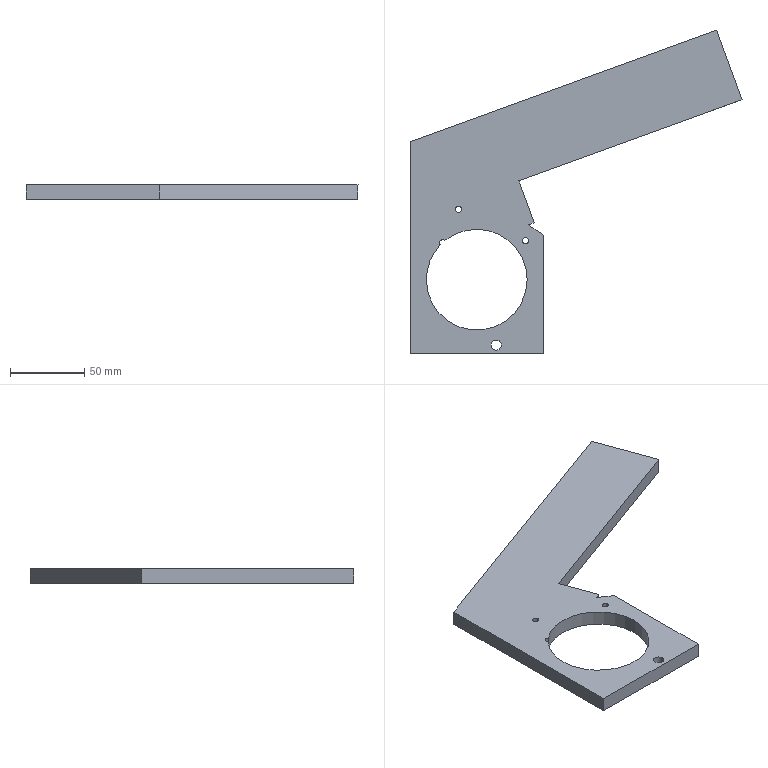Part | SolidWorks | features BaseBody 1 | 1 solid | 21 faces | box 223.833 x 218.263 x 10 mm | volume 168932 mm3 | plane 11 | cylinder 10 | commonest cylinder face diameters 4.2 x5 68 x3 6.8 x2
STEP:
#1=CARTESIAN_POINT('',(212.21,1592.079,-1033.));
#2=VERTEX_POINT('',#1);
#3=CARTESIAN_POINT('',(144.21,1592.079,-1033.));
#4=VERTEX_POINT('',#3);
#5=CARTESIAN_POINT('',(178.21,1592.079,-1033.));
#6=DIRECTION('',(0.,0.,-1.));
#7=DIRECTION('',(-1.,0.,0.));
#8=AXIS2_PLACEMENT_3D('',#5,#6,#7);
#9=CIRCLE('',#8,34.);
#10=EDGE_CURVE('',#2,#4,#9,.T.);
#11=ORIENTED_EDGE('',*,*,#10,.F.);
#12=CARTESIAN_POINT('',(212.21,1592.079,-1043.));
#13=VERTEX_POINT('',#12);
#14=CARTESIAN_POINT('',(212.21,1592.079,-936.833));
#15=DIRECTION('',(0.,0.,-1.));
#16=VECTOR('',#15,1000.);
#17=LINE('',#14,#16);
#18=EDGE_CURVE('',#2,#13,#17,.T.);
#19=ORIENTED_EDGE('',*,*,#18,.T.);
#20=CARTESIAN_POINT('',(144.21,1592.079,-1043.));
#21=VERTEX_POINT('',#20);
#22=CARTESIAN_POINT('',(178.21,1592.079,-1043.));
#23=DIRECTION('',(0.,0.,-1.));
#24=DIRECTION('',(-1.,0.,0.));
#25=AXIS2_PLACEMENT_3D('',#22,#23,#24);
#26=CIRCLE('',#25,34.);
#27=EDGE_CURVE('',#13,#21,#26,.T.);
#28=ORIENTED_EDGE('',*,*,#27,.T.);
#29=CARTESIAN_POINT('',(144.21,1592.079,-936.833));
#30=DIRECTION('',(0.,0.,-1.));
#31=VECTOR('',#30,1000.);
#32=LINE('',#29,#31);
#33=EDGE_CURVE('',#4,#21,#32,.T.);
#34=ORIENTED_EDGE('',*,*,#33,.F.);
#35=EDGE_LOOP('',(#11,#19,#28,#34));
#36=FACE_OUTER_BOUND('',#35,.T.);
#37=CARTESIAN_POINT('',(178.21,1592.079,-936.833));
#38=DIRECTION('',(0.,0.,-1.));
#39=DIRECTION('',(-1.,0.,0.));
#40=AXIS2_PLACEMENT_3D('',#37,#38,#39);
#41=CYLINDRICAL_SURFACE('',#40,34.);
#42=ADVANCED_FACE('',(#36),#41,.F.);
#43=CARTESIAN_POINT('',(153.644,1615.584,-1033.));
#44=VERTEX_POINT('',#43);
#45=CARTESIAN_POINT('',(178.21,1592.079,-1033.));
#46=DIRECTION('',(0.,0.,-1.));
#47=DIRECTION('',(-1.,0.,0.));
#48=AXIS2_PLACEMENT_3D('',#45,#46,#47);
#49=CIRCLE('',#48,34.);
#50=EDGE_CURVE('',#4,#44,#49,.T.);
#51=ORIENTED_EDGE('',*,*,#50,.F.);
#52=ORIENTED_EDGE('',*,*,#33,.T.);
#53=CARTESIAN_POINT('',(153.644,1615.584,-1043.));
#54=VERTEX_POINT('',#53);
#55=CARTESIAN_POINT('',(178.21,1592.079,-1043.));
#56=DIRECTION('',(0.,0.,-1.));
#57=DIRECTION('',(-1.,0.,0.));
#58=AXIS2_PLACEMENT_3D('',#55,#56,#57);
#59=CIRCLE('',#58,34.);
#60=EDGE_CURVE('',#21,#54,#59,.T.);
#61=ORIENTED_EDGE('',*,*,#60,.T.);
#62=CARTESIAN_POINT('',(153.644,1615.584,-1033.));
#63=DIRECTION('',(0.,0.,1.));
#64=VECTOR('',#63,1000.);
#65=LINE('',#62,#64);
#66=EDGE_CURVE('',#54,#44,#65,.T.);
#67=ORIENTED_EDGE('',*,*,#66,.T.);
#68=EDGE_LOOP('',(#51,#52,#61,#67));
#69=FACE_OUTER_BOUND('',#68,.T.);
#70=CARTESIAN_POINT('',(178.21,1592.079,-936.833));
#71=DIRECTION('',(0.,0.,-1.));
#72=DIRECTION('',(-1.,0.,0.));
#73=AXIS2_PLACEMENT_3D('',#70,#71,#72);
#74=CYLINDRICAL_SURFACE('',#73,34.);
#75=ADVANCED_FACE('',(#69),#74,.F.);
#76=CARTESIAN_POINT('',(194.715,1547.971,-1043.));
#77=VERTEX_POINT('',#76);
#78=CARTESIAN_POINT('',(187.915,1547.971,-1043.));
#79=VERTEX_POINT('',#78);
#80=CARTESIAN_POINT('',(191.315,1547.971,-1043.));
#81=DIRECTION('',(0.,0.,-1.));
#82=DIRECTION('',(1.,0.,0.));
#83=AXIS2_PLACEMENT_3D('',#80,#81,#82);
#84=CIRCLE('',#83,3.4);
#85=EDGE_CURVE('',#77,#79,#84,.T.);
#86=ORIENTED_EDGE('',*,*,#85,.T.);
#87=CARTESIAN_POINT('',(187.915,1547.971,-1033.));
#88=VERTEX_POINT('',#87);
#89=CARTESIAN_POINT('',(187.915,1547.971,-1033.));
#90=DIRECTION('',(0.,0.,1.));
#91=VECTOR('',#90,1000.);
#92=LINE('',#89,#91);
#93=EDGE_CURVE('',#79,#88,#92,.T.);
#94=ORIENTED_EDGE('',*,*,#93,.T.);
#95=CARTESIAN_POINT('',(194.715,1547.971,-1033.));
#96=VERTEX_POINT('',#95);
#97=CARTESIAN_POINT('',(191.315,1547.971,-1033.));
#98=DIRECTION('',(0.,0.,-1.));
#99=DIRECTION('',(1.,0.,0.));
#100=AXIS2_PLACEMENT_3D('',#97,#98,#99);
#101=CIRCLE('',#100,3.4);
#102=EDGE_CURVE('',#96,#88,#101,.T.);
#103=ORIENTED_EDGE('',*,*,#102,.F.);
#104=CARTESIAN_POINT('',(194.715,1547.971,-1033.));
#105=DIRECTION('',(0.,0.,1.));
#106=VECTOR('',#105,1000.);
#107=LINE('',#104,#106);
#108=EDGE_CURVE('',#77,#96,#107,.T.);
#109=ORIENTED_EDGE('',*,*,#108,.F.);
#110=EDGE_LOOP('',(#86,#94,#103,#109));
#111=FACE_OUTER_BOUND('',#110,.T.);
#112=CARTESIAN_POINT('',(191.315,1547.971,-1033.));
#113=DIRECTION('',(0.,0.,1.));
#114=DIRECTION('',(1.,0.,0.));
#115=AXIS2_PLACEMENT_3D('',#112,#113,#114);
#116=CYLINDRICAL_SURFACE('',#115,3.4);
#117=ADVANCED_FACE('',(#111),#116,.F.);
#118=CARTESIAN_POINT('',(167.934,1639.572,-1043.));
#119=VERTEX_POINT('',#118);
#120=CARTESIAN_POINT('',(163.734,1639.572,-1043.));
#121=VERTEX_POINT('',#120);
#122=CARTESIAN_POINT('',(165.834,1639.572,-1043.));
#123=DIRECTION('',(0.,0.,-1.));
#124=DIRECTION('',(1.,0.,0.));
#125=AXIS2_PLACEMENT_3D('',#122,#123,#124);
#126=CIRCLE('',#125,2.1);
#127=EDGE_CURVE('',#119,#121,#126,.T.);
#128=ORIENTED_EDGE('',*,*,#127,.T.);
#129=CARTESIAN_POINT('',(163.734,1639.572,-1033.));
#130=VERTEX_POINT('',#129);
#131=CARTESIAN_POINT('',(163.734,1639.572,-1033.));
#132=DIRECTION('',(0.,0.,1.));
#133=VECTOR('',#132,1000.);
#134=LINE('',#131,#133);
#135=EDGE_CURVE('',#121,#130,#134,.T.);
#136=ORIENTED_EDGE('',*,*,#135,.T.);
#137=CARTESIAN_POINT('',(167.934,1639.572,-1033.));
#138=VERTEX_POINT('',#137);
#139=CARTESIAN_POINT('',(165.834,1639.572,-1033.));
#140=DIRECTION('',(0.,0.,-1.));
#141=DIRECTION('',(1.,0.,0.));
#142=AXIS2_PLACEMENT_3D('',#139,#140,#141);
#143=CIRCLE('',#142,2.1);
#144=EDGE_CURVE('',#138,#130,#143,.T.);
#145=ORIENTED_EDGE('',*,*,#144,.F.);
#146=CARTESIAN_POINT('',(167.934,1639.572,-1033.));
#147=DIRECTION('',(0.,0.,1.));
#148=VECTOR('',#147,1000.);
#149=LINE('',#146,#148);
#150=EDGE_CURVE('',#119,#138,#149,.T.);
#151=ORIENTED_EDGE('',*,*,#150,.F.);
#152=EDGE_LOOP('',(#128,#136,#145,#151));
#153=FACE_OUTER_BOUND('',#152,.T.);
#154=CARTESIAN_POINT('',(165.834,1639.572,-1033.));
#155=DIRECTION('',(0.,0.,1.));
#156=DIRECTION('',(1.,0.,0.));
#157=AXIS2_PLACEMENT_3D('',#154,#155,#156);
#158=CYLINDRICAL_SURFACE('',#157,2.1);
#159=ADVANCED_FACE('',(#153),#158,.F.);
#160=CARTESIAN_POINT('',(213.25,1618.441,-1043.));
#161=VERTEX_POINT('',#160);
#162=CARTESIAN_POINT('',(209.05,1618.441,-1043.));
#163=VERTEX_POINT('',#162);
#164=CARTESIAN_POINT('',(211.15,1618.441,-1043.));
#165=DIRECTION('',(0.,0.,-1.));
#166=DIRECTION('',(1.,0.,0.));
#167=AXIS2_PLACEMENT_3D('',#164,#165,#166);
#168=CIRCLE('',#167,2.1);
#169=EDGE_CURVE('',#161,#163,#168,.T.);
#170=ORIENTED_EDGE('',*,*,#169,.T.);
#171=CARTESIAN_POINT('',(209.05,1618.441,-1033.));
#172=VERTEX_POINT('',#171);
#173=CARTESIAN_POINT('',(209.05,1618.441,-1033.));
#174=DIRECTION('',(0.,0.,1.));
#175=VECTOR('',#174,1000.);
#176=LINE('',#173,#175);
#177=EDGE_CURVE('',#163,#172,#176,.T.);
#178=ORIENTED_EDGE('',*,*,#177,.T.);
#179=CARTESIAN_POINT('',(213.25,1618.441,-1033.));
#180=VERTEX_POINT('',#179);
#181=CARTESIAN_POINT('',(211.15,1618.441,-1033.));
#182=DIRECTION('',(0.,0.,-1.));
#183=DIRECTION('',(1.,0.,0.));
#184=AXIS2_PLACEMENT_3D('',#181,#182,#183);
#185=CIRCLE('',#184,2.1);
#186=EDGE_CURVE('',#180,#172,#185,.T.);
#187=ORIENTED_EDGE('',*,*,#186,.F.);
#188=CARTESIAN_POINT('',(213.25,1618.441,-1033.));
#189=DIRECTION('',(0.,0.,1.));
#190=VECTOR('',#189,1000.);
#191=LINE('',#188,#190);
#192=EDGE_CURVE('',#161,#180,#191,.T.);
#193=ORIENTED_EDGE('',*,*,#192,.F.);
#194=EDGE_LOOP('',(#170,#178,#187,#193));
#195=FACE_OUTER_BOUND('',#194,.T.);
#196=CARTESIAN_POINT('',(211.15,1618.441,-1033.));
#197=DIRECTION('',(0.,0.,1.));
#198=DIRECTION('',(1.,0.,0.));
#199=AXIS2_PLACEMENT_3D('',#196,#197,#198);
#200=CYLINDRICAL_SURFACE('',#199,2.1);
#201=ADVANCED_FACE('',(#195),#200,.F.);
#202=CARTESIAN_POINT('',(156.724,1618.429,-1043.));
#203=VERTEX_POINT('',#202);
#204=CARTESIAN_POINT('',(178.21,1592.079,-1043.));
#205=DIRECTION('',(0.,0.,-1.));
#206=DIRECTION('',(-1.,0.,0.));
#207=AXIS2_PLACEMENT_3D('',#204,#205,#206);
#208=CIRCLE('',#207,34.);
#209=EDGE_CURVE('',#203,#13,#208,.T.);
#210=ORIENTED_EDGE('',*,*,#209,.F.);
#211=CARTESIAN_POINT('',(155.269,1616.915,-1043.));
#212=DIRECTION('',(0.,0.,-1.));
#213=DIRECTION('',(1.,0.,0.));
#214=AXIS2_PLACEMENT_3D('',#211,#212,#213);
#215=CIRCLE('',#214,2.1);
#216=EDGE_CURVE('',#54,#203,#215,.T.);
#217=ORIENTED_EDGE('',*,*,#216,.F.);
#218=ORIENTED_EDGE('',*,*,#60,.F.);
#219=ORIENTED_EDGE('',*,*,#27,.F.);
#220=EDGE_LOOP('',(#210,#217,#218,#219));
#221=FACE_BOUND('',#220,.T.);
#222=ORIENTED_EDGE('',*,*,#85,.F.);
#223=CARTESIAN_POINT('',(191.315,1547.971,-1043.));
#224=DIRECTION('',(0.,0.,-1.));
#225=DIRECTION('',(1.,0.,0.));
#226=AXIS2_PLACEMENT_3D('',#223,#224,#225);
#227=CIRCLE('',#226,3.4);
#228=EDGE_CURVE('',#79,#77,#227,.T.);
#229=ORIENTED_EDGE('',*,*,#228,.F.);
#230=EDGE_LOOP('',(#222,#229));
#231=FACE_BOUND('',#230,.T.);
#232=ORIENTED_EDGE('',*,*,#127,.F.);
#233=CARTESIAN_POINT('',(165.834,1639.572,-1043.));
#234=DIRECTION('',(0.,0.,-1.));
#235=DIRECTION('',(1.,0.,0.));
#236=AXIS2_PLACEMENT_3D('',#233,#234,#235);
#237=CIRCLE('',#236,2.1);
#238=EDGE_CURVE('',#121,#119,#237,.T.);
#239=ORIENTED_EDGE('',*,*,#238,.F.);
#240=EDGE_LOOP('',(#232,#239));
#241=FACE_BOUND('',#240,.T.);
#242=ORIENTED_EDGE('',*,*,#169,.F.);
#243=CARTESIAN_POINT('',(211.15,1618.441,-1043.));
#244=DIRECTION('',(0.,0.,-1.));
#245=DIRECTION('',(1.,0.,0.));
#246=AXIS2_PLACEMENT_3D('',#243,#244,#245);
#247=CIRCLE('',#246,2.1);
#248=EDGE_CURVE('',#163,#161,#247,.T.);
#249=ORIENTED_EDGE('',*,*,#248,.F.);
#250=EDGE_LOOP('',(#242,#249));
#251=FACE_BOUND('',#250,.T.);
#252=CARTESIAN_POINT('',(357.044,1713.357,-1043.));
#253=VERTEX_POINT('',#252);
#254=CARTESIAN_POINT('',(339.943,1760.342,-1043.));
#255=VERTEX_POINT('',#254);
#256=CARTESIAN_POINT('',(357.044,1713.357,-1043.));
#257=DIRECTION('',(-0.342,0.9397,0.));
#258=VECTOR('',#257,1000.);
#259=LINE('',#256,#258);
#260=EDGE_CURVE('',#253,#255,#259,.T.);
#261=ORIENTED_EDGE('',*,*,#260,.F.);
#262=CARTESIAN_POINT('',(206.693,1658.634,-1043.));
#263=VERTEX_POINT('',#262);
#264=CARTESIAN_POINT('',(206.693,1658.634,-1043.));
#265=DIRECTION('',(0.9397,0.342,0.));
#266=VECTOR('',#265,1000.);
#267=LINE('',#264,#266);
#268=EDGE_CURVE('',#263,#253,#267,.T.);
#269=ORIENTED_EDGE('',*,*,#268,.F.);
#270=CARTESIAN_POINT('',(216.953,1630.443,-1043.));
#271=VERTEX_POINT('',#270);
#272=CARTESIAN_POINT('',(216.953,1630.443,-1043.));
#273=DIRECTION('',(-0.342,0.9397,0.));
#274=VECTOR('',#273,1000.);
#275=LINE('',#272,#274);
#276=EDGE_CURVE('',#271,#263,#275,.T.);
#277=ORIENTED_EDGE('',*,*,#276,.F.);
#278=CARTESIAN_POINT('',(213.21,1629.081,-1043.));
#279=VERTEX_POINT('',#278);
#280=CARTESIAN_POINT('',(213.21,1629.081,-1043.));
#281=DIRECTION('',(0.9397,0.342,0.));
#282=VECTOR('',#281,1000.);
#283=LINE('',#280,#282);
#284=EDGE_CURVE('',#279,#271,#283,.T.);
#285=ORIENTED_EDGE('',*,*,#284,.F.);
#286=CARTESIAN_POINT('',(223.21,1622.079,-1043.));
#287=VERTEX_POINT('',#286);
#288=CARTESIAN_POINT('',(223.21,1622.079,-1043.));
#289=DIRECTION('',(-0.8192,0.5736,0.));
#290=VECTOR('',#289,1000.);
#291=LINE('',#288,#290);
#292=EDGE_CURVE('',#287,#279,#291,.T.);
#293=ORIENTED_EDGE('',*,*,#292,.F.);
#294=CARTESIAN_POINT('',(223.21,1542.079,-1043.));
#295=VERTEX_POINT('',#294);
#296=CARTESIAN_POINT('',(223.21,1685.097,-1043.));
#297=DIRECTION('',(0.,1.,0.));
#298=VECTOR('',#297,1000.);
#299=LINE('',#296,#298);
#300=EDGE_CURVE('',#295,#287,#299,.T.);
#301=ORIENTED_EDGE('',*,*,#300,.F.);
#302=CARTESIAN_POINT('',(133.21,1542.079,-1043.));
#303=VERTEX_POINT('',#302);
#304=CARTESIAN_POINT('',(133.21,1542.079,-1043.));
#305=DIRECTION('',(1.,0.,0.));
#306=VECTOR('',#305,1000.);
#307=LINE('',#304,#306);
#308=EDGE_CURVE('',#303,#295,#307,.T.);
#309=ORIENTED_EDGE('',*,*,#308,.F.);
#310=CARTESIAN_POINT('',(133.21,1685.097,-1043.));
#311=VERTEX_POINT('',#310);
#312=CARTESIAN_POINT('',(133.21,1685.097,-1043.));
#313=DIRECTION('',(0.,-1.,0.));
#314=VECTOR('',#313,1000.);
#315=LINE('',#312,#314);
#316=EDGE_CURVE('',#311,#303,#315,.T.);
#317=ORIENTED_EDGE('',*,*,#316,.F.);
#318=CARTESIAN_POINT('',(339.943,1760.342,-1043.));
#319=DIRECTION('',(-0.9397,-0.342,0.));
#320=VECTOR('',#319,1000.);
#321=LINE('',#318,#320);
#322=EDGE_CURVE('',#255,#311,#321,.T.);
#323=ORIENTED_EDGE('',*,*,#322,.F.);
#324=EDGE_LOOP('',(#261,#269,#277,#285,#293,#301,#309,#317,#323));
#325=FACE_OUTER_BOUND('',#324,.T.);
#326=CARTESIAN_POINT('',(133.21,1685.097,-1043.));
#327=DIRECTION('',(0.,0.,1.));
#328=DIRECTION('',(1.,0.,0.));
#329=AXIS2_PLACEMENT_3D('',#326,#327,#328);
#330=PLANE('',#329);
#331=ADVANCED_FACE('',(#221,#231,#241,#251,#325),#330,.F.);
#332=ORIENTED_EDGE('',*,*,#216,.T.);
#333=CARTESIAN_POINT('',(156.724,1618.429,-1033.));
#334=VERTEX_POINT('',#333);
#335=CARTESIAN_POINT('',(156.724,1618.429,-1033.));
#336=DIRECTION('',(0.,0.,-1.));
#337=VECTOR('',#336,1000.);
#338=LINE('',#335,#337);
#339=EDGE_CURVE('',#334,#203,#338,.T.);
#340=ORIENTED_EDGE('',*,*,#339,.F.);
#341=CARTESIAN_POINT('',(155.269,1616.915,-1033.));
#342=DIRECTION('',(0.,0.,-1.));
#343=DIRECTION('',(1.,0.,0.));
#344=AXIS2_PLACEMENT_3D('',#341,#342,#343);
#345=CIRCLE('',#344,2.1);
#346=EDGE_CURVE('',#44,#334,#345,.T.);
#347=ORIENTED_EDGE('',*,*,#346,.F.);
#348=ORIENTED_EDGE('',*,*,#66,.F.);
#349=EDGE_LOOP('',(#332,#340,#347,#348));
#350=FACE_OUTER_BOUND('',#349,.T.);
#351=CARTESIAN_POINT('',(155.269,1616.915,-1033.));
#352=DIRECTION('',(0.,0.,1.));
#353=DIRECTION('',(1.,0.,0.));
#354=AXIS2_PLACEMENT_3D('',#351,#352,#353);
#355=CYLINDRICAL_SURFACE('',#354,2.1);
#356=ADVANCED_FACE('',(#350),#355,.F.);
#357=ORIENTED_EDGE('',*,*,#18,.F.);
#358=CARTESIAN_POINT('',(178.21,1592.079,-1033.));
#359=DIRECTION('',(0.,0.,-1.));
#360=DIRECTION('',(-1.,0.,0.));
#361=AXIS2_PLACEMENT_3D('',#358,#359,#360);
#362=CIRCLE('',#361,34.);
#363=EDGE_CURVE('',#334,#2,#362,.T.);
#364=ORIENTED_EDGE('',*,*,#363,.F.);
#365=ORIENTED_EDGE('',*,*,#339,.T.);
#366=ORIENTED_EDGE('',*,*,#209,.T.);
#367=EDGE_LOOP('',(#357,#364,#365,#366));
#368=FACE_OUTER_BOUND('',#367,.T.);
#369=CARTESIAN_POINT('',(178.21,1592.079,-936.833));
#370=DIRECTION('',(0.,0.,-1.));
#371=DIRECTION('',(-1.,0.,0.));
#372=AXIS2_PLACEMENT_3D('',#369,#370,#371);
#373=CYLINDRICAL_SURFACE('',#372,34.);
#374=ADVANCED_FACE('',(#368),#373,.F.);
#375=ORIENTED_EDGE('',*,*,#93,.F.);
#376=ORIENTED_EDGE('',*,*,#228,.T.);
#377=ORIENTED_EDGE('',*,*,#108,.T.);
#378=CARTESIAN_POINT('',(191.315,1547.971,-1033.));
#379=DIRECTION('',(0.,0.,-1.));
#380=DIRECTION('',(1.,0.,0.));
#381=AXIS2_PLACEMENT_3D('',#378,#379,#380);
#382=CIRCLE('',#381,3.4);
#383=EDGE_CURVE('',#88,#96,#382,.T.);
#384=ORIENTED_EDGE('',*,*,#383,.F.);
#385=EDGE_LOOP('',(#375,#376,#377,#384));
#386=FACE_OUTER_BOUND('',#385,.T.);
#387=CARTESIAN_POINT('',(191.315,1547.971,-1033.));
#388=DIRECTION('',(0.,0.,1.));
#389=DIRECTION('',(1.,0.,0.));
#390=AXIS2_PLACEMENT_3D('',#387,#388,#389);
#391=CYLINDRICAL_SURFACE('',#390,3.4);
#392=ADVANCED_FACE('',(#386),#391,.F.);
#393=ORIENTED_EDGE('',*,*,#135,.F.);
#394=ORIENTED_EDGE('',*,*,#238,.T.);
#395=ORIENTED_EDGE('',*,*,#150,.T.);
#396=CARTESIAN_POINT('',(165.834,1639.572,-1033.));
#397=DIRECTION('',(0.,0.,-1.));
#398=DIRECTION('',(1.,0.,0.));
#399=AXIS2_PLACEMENT_3D('',#396,#397,#398);
#400=CIRCLE('',#399,2.1);
#401=EDGE_CURVE('',#130,#138,#400,.T.);
#402=ORIENTED_EDGE('',*,*,#401,.F.);
#403=EDGE_LOOP('',(#393,#394,#395,#402));
#404=FACE_OUTER_BOUND('',#403,.T.);
#405=CARTESIAN_POINT('',(165.834,1639.572,-1033.));
#406=DIRECTION('',(0.,0.,1.));
#407=DIRECTION('',(1.,0.,0.));
#408=AXIS2_PLACEMENT_3D('',#405,#406,#407);
#409=CYLINDRICAL_SURFACE('',#408,2.1);
#410=ADVANCED_FACE('',(#404),#409,.F.);
#411=ORIENTED_EDGE('',*,*,#177,.F.);
#412=ORIENTED_EDGE('',*,*,#248,.T.);
#413=ORIENTED_EDGE('',*,*,#192,.T.);
#414=CARTESIAN_POINT('',(211.15,1618.441,-1033.));
#415=DIRECTION('',(0.,0.,-1.));
#416=DIRECTION('',(1.,0.,0.));
#417=AXIS2_PLACEMENT_3D('',#414,#415,#416);
#418=CIRCLE('',#417,2.1);
#419=EDGE_CURVE('',#172,#180,#418,.T.);
#420=ORIENTED_EDGE('',*,*,#419,.F.);
#421=EDGE_LOOP('',(#411,#412,#413,#420));
#422=FACE_OUTER_BOUND('',#421,.T.);
#423=CARTESIAN_POINT('',(211.15,1618.441,-1033.));
#424=DIRECTION('',(0.,0.,1.));
#425=DIRECTION('',(1.,0.,0.));
#426=AXIS2_PLACEMENT_3D('',#423,#424,#425);
#427=CYLINDRICAL_SURFACE('',#426,2.1);
#428=ADVANCED_FACE('',(#422),#427,.F.);
#429=ORIENTED_EDGE('',*,*,#322,.T.);
#430=CARTESIAN_POINT('',(133.21,1685.097,-1033.));
#431=VERTEX_POINT('',#430);
#432=CARTESIAN_POINT('',(133.21,1685.097,-933.));
#433=DIRECTION('',(0.,0.,1.));
#434=VECTOR('',#433,1000.);
#435=LINE('',#432,#434);
#436=EDGE_CURVE('',#311,#431,#435,.T.);
#437=ORIENTED_EDGE('',*,*,#436,.T.);
#438=CARTESIAN_POINT('',(339.943,1760.342,-1033.));
#439=VERTEX_POINT('',#438);
#440=CARTESIAN_POINT('',(133.21,1685.097,-1033.));
#441=DIRECTION('',(0.9397,0.342,0.));
#442=VECTOR('',#441,1000.);
#443=LINE('',#440,#442);
#444=EDGE_CURVE('',#431,#439,#443,.T.);
#445=ORIENTED_EDGE('',*,*,#444,.T.);
#446=CARTESIAN_POINT('',(339.943,1760.342,-933.));
#447=DIRECTION('',(0.,0.,-1.));
#448=VECTOR('',#447,1000.);
#449=LINE('',#446,#448);
#450=EDGE_CURVE('',#439,#255,#449,.T.);
#451=ORIENTED_EDGE('',*,*,#450,.T.);
#452=EDGE_LOOP('',(#429,#437,#445,#451));
#453=FACE_OUTER_BOUND('',#452,.T.);
#454=CARTESIAN_POINT('',(133.21,1685.097,-933.));
#455=DIRECTION('',(-0.342,0.9397,0.));
#456=DIRECTION('',(-0.9397,-0.342,0.));
#457=AXIS2_PLACEMENT_3D('',#454,#455,#456);
#458=PLANE('',#457);
#459=ADVANCED_FACE('',(#453),#458,.T.);
#460=ORIENTED_EDGE('',*,*,#260,.T.);
#461=ORIENTED_EDGE('',*,*,#450,.F.);
#462=CARTESIAN_POINT('',(357.044,1713.357,-1033.));
#463=VERTEX_POINT('',#462);
#464=CARTESIAN_POINT('',(339.943,1760.342,-1033.));
#465=DIRECTION('',(0.342,-0.9397,0.));
#466=VECTOR('',#465,1000.);
#467=LINE('',#464,#466);
#468=EDGE_CURVE('',#439,#463,#467,.T.);
#469=ORIENTED_EDGE('',*,*,#468,.T.);
#470=CARTESIAN_POINT('',(357.044,1713.357,-865.369));
#471=DIRECTION('',(0.,0.,-1.));
#472=VECTOR('',#471,1000.);
#473=LINE('',#470,#472);
#474=EDGE_CURVE('',#463,#253,#473,.T.);
#475=ORIENTED_EDGE('',*,*,#474,.T.);
#476=EDGE_LOOP('',(#460,#461,#469,#475));
#477=FACE_OUTER_BOUND('',#476,.T.);
#478=CARTESIAN_POINT('',(339.943,1760.342,-865.369));
#479=DIRECTION('',(0.9397,0.342,0.));
#480=DIRECTION('',(-0.342,0.9397,0.));
#481=AXIS2_PLACEMENT_3D('',#478,#479,#480);
#482=PLANE('',#481);
#483=ADVANCED_FACE('',(#477),#482,.T.);
#484=ORIENTED_EDGE('',*,*,#268,.T.);
#485=ORIENTED_EDGE('',*,*,#474,.F.);
#486=CARTESIAN_POINT('',(206.693,1658.634,-1033.));
#487=VERTEX_POINT('',#486);
#488=CARTESIAN_POINT('',(206.693,1658.634,-1033.));
#489=DIRECTION('',(-0.9397,-0.342,0.));
#490=VECTOR('',#489,1000.);
#491=LINE('',#488,#490);
#492=EDGE_CURVE('',#463,#487,#491,.T.);
#493=ORIENTED_EDGE('',*,*,#492,.T.);
#494=CARTESIAN_POINT('',(206.693,1658.634,-865.369));
#495=DIRECTION('',(0.,0.,-1.));
#496=VECTOR('',#495,1000.);
#497=LINE('',#494,#496);
#498=EDGE_CURVE('',#487,#263,#497,.T.);
#499=ORIENTED_EDGE('',*,*,#498,.T.);
#500=EDGE_LOOP('',(#484,#485,#493,#499));
#501=FACE_OUTER_BOUND('',#500,.T.);
#502=CARTESIAN_POINT('',(206.693,1658.634,-865.369));
#503=DIRECTION('',(0.342,-0.9397,0.));
#504=DIRECTION('',(0.9397,0.342,0.));
#505=AXIS2_PLACEMENT_3D('',#502,#503,#504);
#506=PLANE('',#505);
#507=ADVANCED_FACE('',(#501),#506,.T.);
#508=ORIENTED_EDGE('',*,*,#276,.T.);
#509=ORIENTED_EDGE('',*,*,#498,.F.);
#510=CARTESIAN_POINT('',(216.953,1630.443,-1033.));
#511=VERTEX_POINT('',#510);
#512=CARTESIAN_POINT('',(216.953,1630.443,-1033.));
#513=DIRECTION('',(0.342,-0.9397,0.));
#514=VECTOR('',#513,1000.);
#515=LINE('',#512,#514);
#516=EDGE_CURVE('',#487,#511,#515,.T.);
#517=ORIENTED_EDGE('',*,*,#516,.T.);
#518=CARTESIAN_POINT('',(216.953,1630.443,-933.));
#519=DIRECTION('',(0.,0.,-1.));
#520=VECTOR('',#519,1000.);
#521=LINE('',#518,#520);
#522=EDGE_CURVE('',#511,#271,#521,.T.);
#523=ORIENTED_EDGE('',*,*,#522,.T.);
#524=EDGE_LOOP('',(#508,#509,#517,#523));
#525=FACE_OUTER_BOUND('',#524,.T.);
#526=CARTESIAN_POINT('',(216.953,1630.443,-933.));
#527=DIRECTION('',(0.9397,0.342,0.));
#528=DIRECTION('',(-0.342,0.9397,0.));
#529=AXIS2_PLACEMENT_3D('',#526,#527,#528);
#530=PLANE('',#529);
#531=ADVANCED_FACE('',(#525),#530,.T.);
#532=CARTESIAN_POINT('',(213.21,1629.081,-1033.));
#533=VERTEX_POINT('',#532);
#534=CARTESIAN_POINT('',(194.267,1622.186,-1033.));
#535=DIRECTION('',(-0.9397,-0.342,0.));
#536=VECTOR('',#535,1000.);
#537=LINE('',#534,#536);
#538=EDGE_CURVE('',#511,#533,#537,.T.);
#539=ORIENTED_EDGE('',*,*,#538,.T.);
#540=CARTESIAN_POINT('',(213.21,1629.081,-933.));
#541=DIRECTION('',(0.,0.,-1.));
#542=VECTOR('',#541,1000.);
#543=LINE('',#540,#542);
#544=EDGE_CURVE('',#533,#279,#543,.T.);
#545=ORIENTED_EDGE('',*,*,#544,.T.);
#546=ORIENTED_EDGE('',*,*,#284,.T.);
#547=ORIENTED_EDGE('',*,*,#522,.F.);
#548=EDGE_LOOP('',(#539,#545,#546,#547));
#549=FACE_OUTER_BOUND('',#548,.T.);
#550=CARTESIAN_POINT('',(194.267,1622.186,-933.));
#551=DIRECTION('',(0.342,-0.9397,0.));
#552=DIRECTION('',(0.9397,0.342,0.));
#553=AXIS2_PLACEMENT_3D('',#550,#551,#552);
#554=PLANE('',#553);
#555=ADVANCED_FACE('',(#549),#554,.T.);
#556=CARTESIAN_POINT('',(223.21,1622.079,-1033.));
#557=VERTEX_POINT('',#556);
#558=CARTESIAN_POINT('',(223.21,1622.079,-1033.));
#559=DIRECTION('',(-0.8192,0.5736,0.));
#560=VECTOR('',#559,1000.);
#561=LINE('',#558,#560);
#562=EDGE_CURVE('',#557,#533,#561,.T.);
#563=ORIENTED_EDGE('',*,*,#562,.F.);
#564=CARTESIAN_POINT('',(223.21,1622.079,-1043.));
#565=DIRECTION('',(0.,0.,1.));
#566=VECTOR('',#565,1000.);
#567=LINE('',#564,#566);
#568=EDGE_CURVE('',#287,#557,#567,.T.);
#569=ORIENTED_EDGE('',*,*,#568,.F.);
#570=ORIENTED_EDGE('',*,*,#292,.T.);
#571=ORIENTED_EDGE('',*,*,#544,.F.);
#572=EDGE_LOOP('',(#563,#569,#570,#571));
#573=FACE_OUTER_BOUND('',#572,.T.);
#574=CARTESIAN_POINT('',(223.21,1622.079,-1043.));
#575=DIRECTION('',(-0.5736,-0.8192,0.));
#576=DIRECTION('',(0.8192,-0.5736,0.));
#577=AXIS2_PLACEMENT_3D('',#574,#575,#576);
#578=PLANE('',#577);
#579=ADVANCED_FACE('',(#573),#578,.F.);
#580=ORIENTED_EDGE('',*,*,#300,.T.);
#581=ORIENTED_EDGE('',*,*,#568,.T.);
#582=CARTESIAN_POINT('',(223.21,1542.079,-1033.));
#583=VERTEX_POINT('',#582);
#584=CARTESIAN_POINT('',(223.21,1622.079,-1033.));
#585=DIRECTION('',(0.,1.,0.));
#586=VECTOR('',#585,1000.);
#587=LINE('',#584,#586);
#588=EDGE_CURVE('',#583,#557,#587,.T.);
#589=ORIENTED_EDGE('',*,*,#588,.F.);
#590=CARTESIAN_POINT('',(223.21,1542.079,-1043.));
#591=DIRECTION('',(0.,0.,1.));
#592=VECTOR('',#591,1000.);
#593=LINE('',#590,#592);
#594=EDGE_CURVE('',#295,#583,#593,.T.);
#595=ORIENTED_EDGE('',*,*,#594,.F.);
#596=EDGE_LOOP('',(#580,#581,#589,#595));
#597=FACE_OUTER_BOUND('',#596,.T.);
#598=CARTESIAN_POINT('',(223.21,1622.079,-1043.));
#599=DIRECTION('',(-1.,0.,0.));
#600=DIRECTION('',(0.,0.,1.));
#601=AXIS2_PLACEMENT_3D('',#598,#599,#600);
#602=PLANE('',#601);
#603=ADVANCED_FACE('',(#597),#602,.F.);
#604=ORIENTED_EDGE('',*,*,#308,.T.);
#605=ORIENTED_EDGE('',*,*,#594,.T.);
#606=CARTESIAN_POINT('',(133.21,1542.079,-1033.));
#607=VERTEX_POINT('',#606);
#608=CARTESIAN_POINT('',(223.21,1542.079,-1033.));
#609=DIRECTION('',(1.,0.,0.));
#610=VECTOR('',#609,1000.);
#611=LINE('',#608,#610);
#612=EDGE_CURVE('',#607,#583,#611,.T.);
#613=ORIENTED_EDGE('',*,*,#612,.F.);
#614=CARTESIAN_POINT('',(133.21,1542.079,-1043.));
#615=DIRECTION('',(0.,0.,1.));
#616=VECTOR('',#615,1000.);
#617=LINE('',#614,#616);
#618=EDGE_CURVE('',#303,#607,#617,.T.);
#619=ORIENTED_EDGE('',*,*,#618,.F.);
#620=EDGE_LOOP('',(#604,#605,#613,#619));
#621=FACE_OUTER_BOUND('',#620,.T.);
#622=CARTESIAN_POINT('',(223.21,1542.079,-1043.));
#623=DIRECTION('',(0.,1.,0.));
#624=DIRECTION('',(0.,0.,1.));
#625=AXIS2_PLACEMENT_3D('',#622,#623,#624);
#626=PLANE('',#625);
#627=ADVANCED_FACE('',(#621),#626,.F.);
#628=ORIENTED_EDGE('',*,*,#316,.T.);
#629=ORIENTED_EDGE('',*,*,#618,.T.);
#630=CARTESIAN_POINT('',(133.21,1685.097,-1033.));
#631=DIRECTION('',(0.,-1.,0.));
#632=VECTOR('',#631,1000.);
#633=LINE('',#630,#632);
#634=EDGE_CURVE('',#431,#607,#633,.T.);
#635=ORIENTED_EDGE('',*,*,#634,.F.);
#636=ORIENTED_EDGE('',*,*,#436,.F.);
#637=EDGE_LOOP('',(#628,#629,#635,#636));
#638=FACE_OUTER_BOUND('',#637,.T.);
#639=CARTESIAN_POINT('',(133.21,1685.097,-1043.));
#640=DIRECTION('',(1.,0.,0.));
#641=DIRECTION('',(0.,0.,-1.));
#642=AXIS2_PLACEMENT_3D('',#639,#640,#641);
#643=PLANE('',#642);
#644=ADVANCED_FACE('',(#638),#643,.F.);
#645=ORIENTED_EDGE('',*,*,#102,.T.);
#646=ORIENTED_EDGE('',*,*,#383,.T.);
#647=EDGE_LOOP('',(#645,#646));
#648=FACE_BOUND('',#647,.T.);
#649=ORIENTED_EDGE('',*,*,#144,.T.);
#650=ORIENTED_EDGE('',*,*,#401,.T.);
#651=EDGE_LOOP('',(#649,#650));
#652=FACE_BOUND('',#651,.T.);
#653=ORIENTED_EDGE('',*,*,#363,.T.);
#654=ORIENTED_EDGE('',*,*,#10,.T.);
#655=ORIENTED_EDGE('',*,*,#50,.T.);
#656=ORIENTED_EDGE('',*,*,#346,.T.);
#657=EDGE_LOOP('',(#653,#654,#655,#656));
#658=FACE_BOUND('',#657,.T.);
#659=ORIENTED_EDGE('',*,*,#186,.T.);
#660=ORIENTED_EDGE('',*,*,#419,.T.);
#661=EDGE_LOOP('',(#659,#660));
#662=FACE_BOUND('',#661,.T.);
#663=ORIENTED_EDGE('',*,*,#588,.T.);
#664=ORIENTED_EDGE('',*,*,#562,.T.);
#665=ORIENTED_EDGE('',*,*,#538,.F.);
#666=ORIENTED_EDGE('',*,*,#516,.F.);
#667=ORIENTED_EDGE('',*,*,#492,.F.);
#668=ORIENTED_EDGE('',*,*,#468,.F.);
#669=ORIENTED_EDGE('',*,*,#444,.F.);
#670=ORIENTED_EDGE('',*,*,#634,.T.);
#671=ORIENTED_EDGE('',*,*,#612,.T.);
#672=EDGE_LOOP('',(#663,#664,#665,#666,#667,#668,#669,#670,#671));
#673=FACE_OUTER_BOUND('',#672,.T.);
#674=CARTESIAN_POINT('',(133.21,1685.097,-1033.));
#675=DIRECTION('',(0.,0.,1.));
#676=DIRECTION('',(1.,0.,0.));
#677=AXIS2_PLACEMENT_3D('',#674,#675,#676);
#678=PLANE('',#677);
#679=ADVANCED_FACE('',(#648,#652,#658,#662,#673),#678,.T.);
#680=CLOSED_SHELL('',(#42,#75,#117,#159,#201,#331,#356,#374,#392,#410,#428,#459,#483,#507,#531,#555,#579,#603,#627,#644,#679));
#681=MANIFOLD_SOLID_BREP('',#680);
#682=CARTESIAN_POINT('',(0.,0.,0.));
#683=DIRECTION('',(0.,0.,1.));
#684=DIRECTION('',(1.,0.,0.));
#685=AXIS2_PLACEMENT_3D('',#682,#683,#684);
#686=(LENGTH_UNIT()NAMED_UNIT(*)SI_UNIT(.MILLI.,.METRE.));
#687=UNCERTAINTY_MEASURE_WITH_UNIT(LENGTH_MEASURE(0.00001),#686,'','');
#688=(NAMED_UNIT(*)PLANE_ANGLE_UNIT()SI_UNIT($,.RADIAN.));
#689=(NAMED_UNIT(*)SI_UNIT($,.STERADIAN.)SOLID_ANGLE_UNIT());
#690=(GEOMETRIC_REPRESENTATION_CONTEXT(3)GLOBAL_UNCERTAINTY_ASSIGNED_CONTEXT((#687))GLOBAL_UNIT_ASSIGNED_CONTEXT((#686,#688,#689))REPRESENTATION_CONTEXT('',''));
#691=ADVANCED_BREP_SHAPE_REPRESENTATION('',(#681,#685),#690);